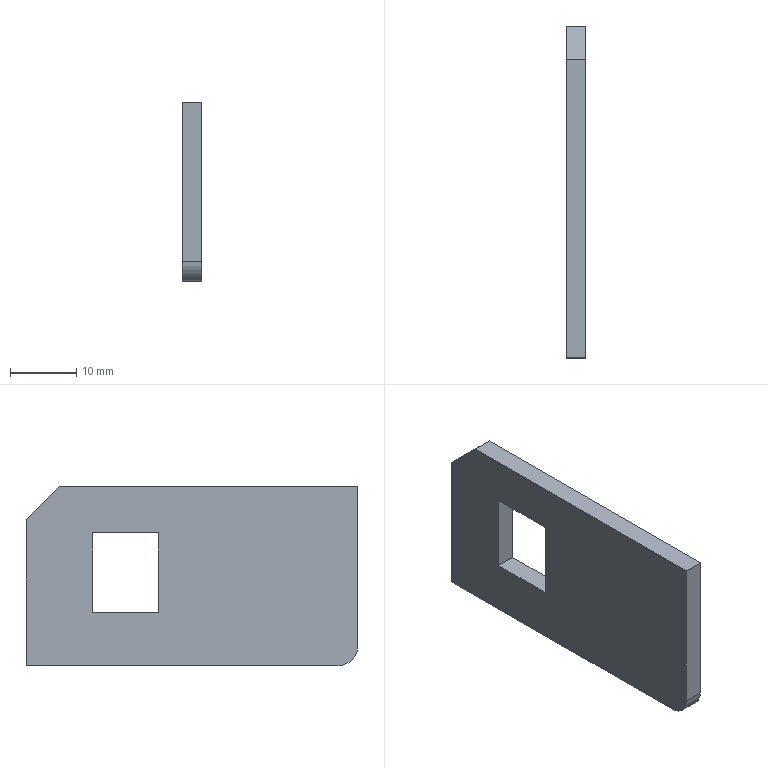Part | SolidWorks | features Cut 1, Extrusion 1, Fillet 1 | 1 solid | 12 faces | box 3 x 50 x 27 mm | volume 3647 mm3 | plane 11 | cylinder 1 | commonest cylinder face diameters 6 x1
STEP:
#1=CARTESIAN_POINT('',(0.,50.,0.));
#2=VERTEX_POINT('',#1);
#3=CARTESIAN_POINT('',(0.,50.,22.));
#4=VERTEX_POINT('',#3);
#5=CARTESIAN_POINT('',(0.,50.,0.));
#6=DIRECTION('',(0.,0.,1.));
#7=VECTOR('',#6,1000.);
#8=LINE('',#5,#7);
#9=EDGE_CURVE('',#2,#4,#8,.T.);
#10=ORIENTED_EDGE('',*,*,#9,.T.);
#11=CARTESIAN_POINT('',(3.,50.,22.));
#12=VERTEX_POINT('',#11);
#13=CARTESIAN_POINT('',(3.,50.,22.));
#14=DIRECTION('',(-1.,0.,0.));
#15=VECTOR('',#14,1000.);
#16=LINE('',#13,#15);
#17=EDGE_CURVE('',#12,#4,#16,.T.);
#18=ORIENTED_EDGE('',*,*,#17,.F.);
#19=CARTESIAN_POINT('',(3.,50.,0.));
#20=VERTEX_POINT('',#19);
#21=CARTESIAN_POINT('',(3.,50.,0.));
#22=DIRECTION('',(0.,0.,1.));
#23=VECTOR('',#22,1000.);
#24=LINE('',#21,#23);
#25=EDGE_CURVE('',#20,#12,#24,.T.);
#26=ORIENTED_EDGE('',*,*,#25,.F.);
#27=CARTESIAN_POINT('',(3.,50.,0.));
#28=DIRECTION('',(-1.,0.,0.));
#29=VECTOR('',#28,1000.);
#30=LINE('',#27,#29);
#31=EDGE_CURVE('',#20,#2,#30,.T.);
#32=ORIENTED_EDGE('',*,*,#31,.T.);
#33=EDGE_LOOP('',(#10,#18,#26,#32));
#34=FACE_OUTER_BOUND('',#33,.T.);
#35=CARTESIAN_POINT('',(3.,50.,0.));
#36=DIRECTION('',(0.,-1.,0.));
#37=DIRECTION('',(0.,0.,-1.));
#38=AXIS2_PLACEMENT_3D('',#35,#36,#37);
#39=PLANE('',#38);
#40=ADVANCED_FACE('',(#34),#39,.F.);
#41=CARTESIAN_POINT('',(0.,45.,27.));
#42=VERTEX_POINT('',#41);
#43=CARTESIAN_POINT('',(0.,50.,22.));
#44=DIRECTION('',(0.,-0.7071,0.7071));
#45=VECTOR('',#44,1000.);
#46=LINE('',#43,#45);
#47=EDGE_CURVE('',#4,#42,#46,.T.);
#48=ORIENTED_EDGE('',*,*,#47,.T.);
#49=CARTESIAN_POINT('',(3.,45.,27.));
#50=VERTEX_POINT('',#49);
#51=CARTESIAN_POINT('',(3.,45.,27.));
#52=DIRECTION('',(-1.,0.,0.));
#53=VECTOR('',#52,1000.);
#54=LINE('',#51,#53);
#55=EDGE_CURVE('',#50,#42,#54,.T.);
#56=ORIENTED_EDGE('',*,*,#55,.F.);
#57=CARTESIAN_POINT('',(3.,50.,22.));
#58=DIRECTION('',(0.,-0.7071,0.7071));
#59=VECTOR('',#58,1000.);
#60=LINE('',#57,#59);
#61=EDGE_CURVE('',#12,#50,#60,.T.);
#62=ORIENTED_EDGE('',*,*,#61,.F.);
#63=ORIENTED_EDGE('',*,*,#17,.T.);
#64=EDGE_LOOP('',(#48,#56,#62,#63));
#65=FACE_OUTER_BOUND('',#64,.T.);
#66=CARTESIAN_POINT('',(3.,50.,22.));
#67=DIRECTION('',(0.,-0.7071,-0.7071));
#68=DIRECTION('',(0.,0.7071,-0.7071));
#69=AXIS2_PLACEMENT_3D('',#66,#67,#68);
#70=PLANE('',#69);
#71=ADVANCED_FACE('',(#65),#70,.F.);
#72=CARTESIAN_POINT('',(0.,0.,27.));
#73=VERTEX_POINT('',#72);
#74=CARTESIAN_POINT('',(0.,45.,27.));
#75=DIRECTION('',(0.,-1.,0.));
#76=VECTOR('',#75,1000.);
#77=LINE('',#74,#76);
#78=EDGE_CURVE('',#42,#73,#77,.T.);
#79=ORIENTED_EDGE('',*,*,#78,.T.);
#80=CARTESIAN_POINT('',(3.,0.,27.));
#81=VERTEX_POINT('',#80);
#82=CARTESIAN_POINT('',(3.,0.,27.));
#83=DIRECTION('',(-1.,0.,0.));
#84=VECTOR('',#83,1000.);
#85=LINE('',#82,#84);
#86=EDGE_CURVE('',#81,#73,#85,.T.);
#87=ORIENTED_EDGE('',*,*,#86,.F.);
#88=CARTESIAN_POINT('',(3.,45.,27.));
#89=DIRECTION('',(0.,-1.,0.));
#90=VECTOR('',#89,1000.);
#91=LINE('',#88,#90);
#92=EDGE_CURVE('',#50,#81,#91,.T.);
#93=ORIENTED_EDGE('',*,*,#92,.F.);
#94=ORIENTED_EDGE('',*,*,#55,.T.);
#95=EDGE_LOOP('',(#79,#87,#93,#94));
#96=FACE_OUTER_BOUND('',#95,.T.);
#97=CARTESIAN_POINT('',(3.,45.,27.));
#98=DIRECTION('',(0.,0.,-1.));
#99=DIRECTION('',(0.,1.,0.));
#100=AXIS2_PLACEMENT_3D('',#97,#98,#99);
#101=PLANE('',#100);
#102=ADVANCED_FACE('',(#96),#101,.F.);
#103=CARTESIAN_POINT('',(0.,0.,3.));
#104=VERTEX_POINT('',#103);
#105=CARTESIAN_POINT('',(0.,0.,27.));
#106=DIRECTION('',(0.,0.,-1.));
#107=VECTOR('',#106,1000.);
#108=LINE('',#105,#107);
#109=EDGE_CURVE('',#73,#104,#108,.T.);
#110=ORIENTED_EDGE('',*,*,#109,.T.);
#111=CARTESIAN_POINT('',(3.,0.,3.));
#112=VERTEX_POINT('',#111);
#113=CARTESIAN_POINT('',(3.,0.,3.));
#114=DIRECTION('',(1.,0.,0.));
#115=VECTOR('',#114,1000.);
#116=LINE('',#113,#115);
#117=EDGE_CURVE('',#104,#112,#116,.T.);
#118=ORIENTED_EDGE('',*,*,#117,.T.);
#119=CARTESIAN_POINT('',(3.,0.,27.));
#120=DIRECTION('',(0.,0.,-1.));
#121=VECTOR('',#120,1000.);
#122=LINE('',#119,#121);
#123=EDGE_CURVE('',#81,#112,#122,.T.);
#124=ORIENTED_EDGE('',*,*,#123,.F.);
#125=ORIENTED_EDGE('',*,*,#86,.T.);
#126=EDGE_LOOP('',(#110,#118,#124,#125));
#127=FACE_OUTER_BOUND('',#126,.T.);
#128=CARTESIAN_POINT('',(3.,0.,27.));
#129=DIRECTION('',(0.,1.,0.));
#130=DIRECTION('',(0.,0.,1.));
#131=AXIS2_PLACEMENT_3D('',#128,#129,#130);
#132=PLANE('',#131);
#133=ADVANCED_FACE('',(#127),#132,.F.);
#134=CARTESIAN_POINT('',(3.,3.,0.));
#135=VERTEX_POINT('',#134);
#136=CARTESIAN_POINT('',(3.,0.,0.));
#137=DIRECTION('',(0.,1.,0.));
#138=VECTOR('',#137,1000.);
#139=LINE('',#136,#138);
#140=EDGE_CURVE('',#135,#20,#139,.T.);
#141=ORIENTED_EDGE('',*,*,#140,.F.);
#142=CARTESIAN_POINT('',(0.,3.,0.));
#143=VERTEX_POINT('',#142);
#144=CARTESIAN_POINT('',(3.,3.,0.));
#145=DIRECTION('',(-1.,0.,0.));
#146=VECTOR('',#145,1000.);
#147=LINE('',#144,#146);
#148=EDGE_CURVE('',#135,#143,#147,.T.);
#149=ORIENTED_EDGE('',*,*,#148,.T.);
#150=CARTESIAN_POINT('',(0.,0.,0.));
#151=DIRECTION('',(0.,1.,0.));
#152=VECTOR('',#151,1000.);
#153=LINE('',#150,#152);
#154=EDGE_CURVE('',#143,#2,#153,.T.);
#155=ORIENTED_EDGE('',*,*,#154,.T.);
#156=ORIENTED_EDGE('',*,*,#31,.F.);
#157=EDGE_LOOP('',(#141,#149,#155,#156));
#158=FACE_OUTER_BOUND('',#157,.T.);
#159=CARTESIAN_POINT('',(3.,0.,0.));
#160=DIRECTION('',(0.,0.,1.));
#161=DIRECTION('',(1.,0.,0.));
#162=AXIS2_PLACEMENT_3D('',#159,#160,#161);
#163=PLANE('',#162);
#164=ADVANCED_FACE('',(#158),#163,.F.);
#165=CARTESIAN_POINT('',(3.,40.,20.));
#166=VERTEX_POINT('',#165);
#167=CARTESIAN_POINT('',(3.,30.,20.));
#168=VERTEX_POINT('',#167);
#169=CARTESIAN_POINT('',(3.,30.,20.));
#170=DIRECTION('',(0.,-1.,0.));
#171=VECTOR('',#170,1000.);
#172=LINE('',#169,#171);
#173=EDGE_CURVE('',#166,#168,#172,.T.);
#174=ORIENTED_EDGE('',*,*,#173,.F.);
#175=CARTESIAN_POINT('',(3.,40.,8.));
#176=VERTEX_POINT('',#175);
#177=CARTESIAN_POINT('',(3.,40.,20.));
#178=DIRECTION('',(0.,0.,1.));
#179=VECTOR('',#178,1000.);
#180=LINE('',#177,#179);
#181=EDGE_CURVE('',#176,#166,#180,.T.);
#182=ORIENTED_EDGE('',*,*,#181,.F.);
#183=CARTESIAN_POINT('',(3.,30.,8.));
#184=VERTEX_POINT('',#183);
#185=CARTESIAN_POINT('',(3.,30.,8.));
#186=DIRECTION('',(0.,1.,0.));
#187=VECTOR('',#186,1000.);
#188=LINE('',#185,#187);
#189=EDGE_CURVE('',#184,#176,#188,.T.);
#190=ORIENTED_EDGE('',*,*,#189,.F.);
#191=CARTESIAN_POINT('',(3.,30.,20.));
#192=DIRECTION('',(0.,0.,-1.));
#193=VECTOR('',#192,1000.);
#194=LINE('',#191,#193);
#195=EDGE_CURVE('',#168,#184,#194,.T.);
#196=ORIENTED_EDGE('',*,*,#195,.F.);
#197=EDGE_LOOP('',(#174,#182,#190,#196));
#198=FACE_BOUND('',#197,.T.);
#199=ORIENTED_EDGE('',*,*,#123,.T.);
#200=CARTESIAN_POINT('',(3.,3.,3.));
#201=DIRECTION('',(1.,0.,0.));
#202=DIRECTION('',(0.,0.,-1.));
#203=AXIS2_PLACEMENT_3D('',#200,#201,#202);
#204=CIRCLE('',#203,3.);
#205=EDGE_CURVE('',#112,#135,#204,.T.);
#206=ORIENTED_EDGE('',*,*,#205,.T.);
#207=ORIENTED_EDGE('',*,*,#140,.T.);
#208=ORIENTED_EDGE('',*,*,#25,.T.);
#209=ORIENTED_EDGE('',*,*,#61,.T.);
#210=ORIENTED_EDGE('',*,*,#92,.T.);
#211=EDGE_LOOP('',(#199,#206,#207,#208,#209,#210));
#212=FACE_OUTER_BOUND('',#211,.T.);
#213=CARTESIAN_POINT('',(3.,0.,0.));
#214=DIRECTION('',(1.,0.,0.));
#215=DIRECTION('',(0.,0.,-1.));
#216=AXIS2_PLACEMENT_3D('',#213,#214,#215);
#217=PLANE('',#216);
#218=ADVANCED_FACE('',(#198,#212),#217,.T.);
#219=CARTESIAN_POINT('',(0.,40.,8.));
#220=VERTEX_POINT('',#219);
#221=CARTESIAN_POINT('',(0.,40.,20.));
#222=VERTEX_POINT('',#221);
#223=CARTESIAN_POINT('',(0.,40.,20.));
#224=DIRECTION('',(0.,0.,1.));
#225=VECTOR('',#224,1000.);
#226=LINE('',#223,#225);
#227=EDGE_CURVE('',#220,#222,#226,.T.);
#228=ORIENTED_EDGE('',*,*,#227,.T.);
#229=CARTESIAN_POINT('',(0.,30.,20.));
#230=VERTEX_POINT('',#229);
#231=CARTESIAN_POINT('',(0.,30.,20.));
#232=DIRECTION('',(0.,-1.,0.));
#233=VECTOR('',#232,1000.);
#234=LINE('',#231,#233);
#235=EDGE_CURVE('',#222,#230,#234,.T.);
#236=ORIENTED_EDGE('',*,*,#235,.T.);
#237=CARTESIAN_POINT('',(0.,30.,8.));
#238=VERTEX_POINT('',#237);
#239=CARTESIAN_POINT('',(0.,30.,20.));
#240=DIRECTION('',(0.,0.,-1.));
#241=VECTOR('',#240,1000.);
#242=LINE('',#239,#241);
#243=EDGE_CURVE('',#230,#238,#242,.T.);
#244=ORIENTED_EDGE('',*,*,#243,.T.);
#245=CARTESIAN_POINT('',(0.,30.,8.));
#246=DIRECTION('',(0.,1.,0.));
#247=VECTOR('',#246,1000.);
#248=LINE('',#245,#247);
#249=EDGE_CURVE('',#238,#220,#248,.T.);
#250=ORIENTED_EDGE('',*,*,#249,.T.);
#251=EDGE_LOOP('',(#228,#236,#244,#250));
#252=FACE_BOUND('',#251,.T.);
#253=ORIENTED_EDGE('',*,*,#154,.F.);
#254=CARTESIAN_POINT('',(0.,3.,3.));
#255=DIRECTION('',(-1.,0.,0.));
#256=DIRECTION('',(0.,0.,-1.));
#257=AXIS2_PLACEMENT_3D('',#254,#255,#256);
#258=CIRCLE('',#257,3.);
#259=EDGE_CURVE('',#143,#104,#258,.T.);
#260=ORIENTED_EDGE('',*,*,#259,.T.);
#261=ORIENTED_EDGE('',*,*,#109,.F.);
#262=ORIENTED_EDGE('',*,*,#78,.F.);
#263=ORIENTED_EDGE('',*,*,#47,.F.);
#264=ORIENTED_EDGE('',*,*,#9,.F.);
#265=EDGE_LOOP('',(#253,#260,#261,#262,#263,#264));
#266=FACE_OUTER_BOUND('',#265,.T.);
#267=CARTESIAN_POINT('',(0.,0.,0.));
#268=DIRECTION('',(1.,0.,0.));
#269=DIRECTION('',(0.,0.,-1.));
#270=AXIS2_PLACEMENT_3D('',#267,#268,#269);
#271=PLANE('',#270);
#272=ADVANCED_FACE('',(#252,#266),#271,.F.);
#273=ORIENTED_EDGE('',*,*,#205,.F.);
#274=ORIENTED_EDGE('',*,*,#117,.F.);
#275=ORIENTED_EDGE('',*,*,#259,.F.);
#276=ORIENTED_EDGE('',*,*,#148,.F.);
#277=EDGE_LOOP('',(#273,#274,#275,#276));
#278=FACE_OUTER_BOUND('',#277,.T.);
#279=CARTESIAN_POINT('',(3.,3.,3.));
#280=DIRECTION('',(-1.,0.,0.));
#281=DIRECTION('',(0.,0.,1.));
#282=AXIS2_PLACEMENT_3D('',#279,#280,#281);
#283=CYLINDRICAL_SURFACE('',#282,3.);
#284=ADVANCED_FACE('',(#278),#283,.T.);
#285=ORIENTED_EDGE('',*,*,#173,.T.);
#286=CARTESIAN_POINT('',(0.,30.,20.));
#287=DIRECTION('',(1.,0.,0.));
#288=VECTOR('',#287,1000.);
#289=LINE('',#286,#288);
#290=EDGE_CURVE('',#230,#168,#289,.T.);
#291=ORIENTED_EDGE('',*,*,#290,.F.);
#292=ORIENTED_EDGE('',*,*,#235,.F.);
#293=CARTESIAN_POINT('',(0.,40.,20.));
#294=DIRECTION('',(1.,0.,0.));
#295=VECTOR('',#294,1000.);
#296=LINE('',#293,#295);
#297=EDGE_CURVE('',#222,#166,#296,.T.);
#298=ORIENTED_EDGE('',*,*,#297,.T.);
#299=EDGE_LOOP('',(#285,#291,#292,#298));
#300=FACE_OUTER_BOUND('',#299,.T.);
#301=CARTESIAN_POINT('',(0.,30.,20.));
#302=DIRECTION('',(0.,0.,1.));
#303=DIRECTION('',(1.,0.,0.));
#304=AXIS2_PLACEMENT_3D('',#301,#302,#303);
#305=PLANE('',#304);
#306=ADVANCED_FACE('',(#300),#305,.F.);
#307=ORIENTED_EDGE('',*,*,#181,.T.);
#308=ORIENTED_EDGE('',*,*,#297,.F.);
#309=ORIENTED_EDGE('',*,*,#227,.F.);
#310=CARTESIAN_POINT('',(0.,40.,8.));
#311=DIRECTION('',(1.,0.,0.));
#312=VECTOR('',#311,1000.);
#313=LINE('',#310,#312);
#314=EDGE_CURVE('',#220,#176,#313,.T.);
#315=ORIENTED_EDGE('',*,*,#314,.T.);
#316=EDGE_LOOP('',(#307,#308,#309,#315));
#317=FACE_OUTER_BOUND('',#316,.T.);
#318=CARTESIAN_POINT('',(0.,40.,20.));
#319=DIRECTION('',(0.,1.,0.));
#320=DIRECTION('',(0.,0.,1.));
#321=AXIS2_PLACEMENT_3D('',#318,#319,#320);
#322=PLANE('',#321);
#323=ADVANCED_FACE('',(#317),#322,.F.);
#324=ORIENTED_EDGE('',*,*,#189,.T.);
#325=ORIENTED_EDGE('',*,*,#314,.F.);
#326=ORIENTED_EDGE('',*,*,#249,.F.);
#327=CARTESIAN_POINT('',(0.,30.,8.));
#328=DIRECTION('',(1.,0.,0.));
#329=VECTOR('',#328,1000.);
#330=LINE('',#327,#329);
#331=EDGE_CURVE('',#238,#184,#330,.T.);
#332=ORIENTED_EDGE('',*,*,#331,.T.);
#333=EDGE_LOOP('',(#324,#325,#326,#332));
#334=FACE_OUTER_BOUND('',#333,.T.);
#335=CARTESIAN_POINT('',(0.,30.,8.));
#336=DIRECTION('',(0.,0.,-1.));
#337=DIRECTION('',(-1.,0.,0.));
#338=AXIS2_PLACEMENT_3D('',#335,#336,#337);
#339=PLANE('',#338);
#340=ADVANCED_FACE('',(#334),#339,.F.);
#341=ORIENTED_EDGE('',*,*,#195,.T.);
#342=ORIENTED_EDGE('',*,*,#331,.F.);
#343=ORIENTED_EDGE('',*,*,#243,.F.);
#344=ORIENTED_EDGE('',*,*,#290,.T.);
#345=EDGE_LOOP('',(#341,#342,#343,#344));
#346=FACE_OUTER_BOUND('',#345,.T.);
#347=CARTESIAN_POINT('',(0.,30.,20.));
#348=DIRECTION('',(0.,-1.,0.));
#349=DIRECTION('',(0.,0.,-1.));
#350=AXIS2_PLACEMENT_3D('',#347,#348,#349);
#351=PLANE('',#350);
#352=ADVANCED_FACE('',(#346),#351,.F.);
#353=CLOSED_SHELL('',(#40,#71,#102,#133,#164,#218,#272,#284,#306,#323,#340,#352));
#354=MANIFOLD_SOLID_BREP('',#353);
#355=CARTESIAN_POINT('',(0.,0.,0.));
#356=DIRECTION('',(0.,0.,1.));
#357=DIRECTION('',(1.,0.,0.));
#358=AXIS2_PLACEMENT_3D('',#355,#356,#357);
#359=(LENGTH_UNIT()NAMED_UNIT(*)SI_UNIT(.MILLI.,.METRE.));
#360=UNCERTAINTY_MEASURE_WITH_UNIT(LENGTH_MEASURE(0.00001),#359,'','');
#361=(NAMED_UNIT(*)PLANE_ANGLE_UNIT()SI_UNIT($,.RADIAN.));
#362=(NAMED_UNIT(*)SI_UNIT($,.STERADIAN.)SOLID_ANGLE_UNIT());
#363=(GEOMETRIC_REPRESENTATION_CONTEXT(3)GLOBAL_UNCERTAINTY_ASSIGNED_CONTEXT((#360))GLOBAL_UNIT_ASSIGNED_CONTEXT((#359,#361,#362))REPRESENTATION_CONTEXT('',''));
#364=ADVANCED_BREP_SHAPE_REPRESENTATION('',(#354,#358),#363);